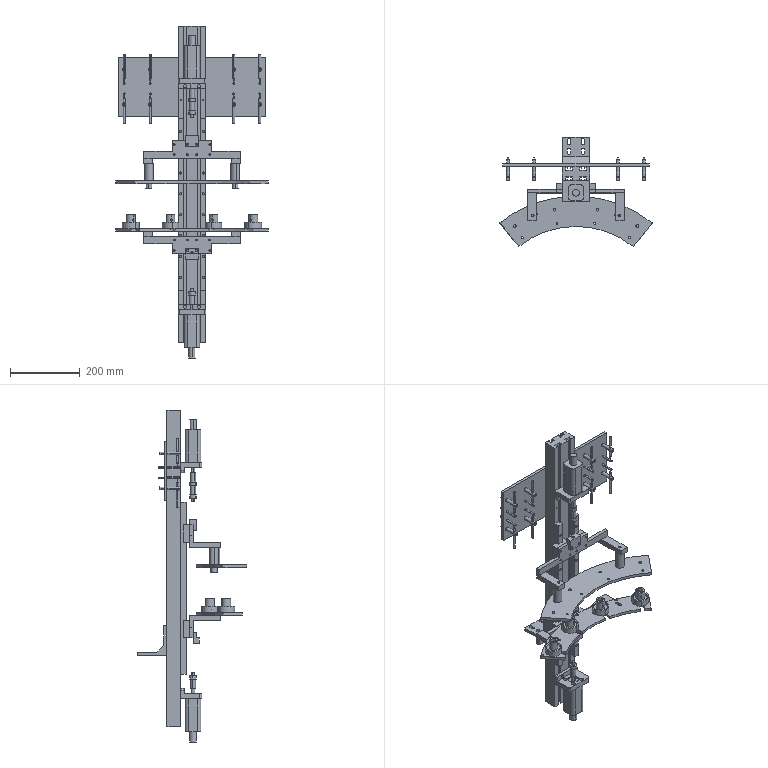Part | 54 solids | 1135 faces | box 437.882 x 314.149 x 954 mm | volume 4931479 mm3 | cylinder 648 | plane 369 | cone 118 | commonest cylinder face diameters 5 x96 3.3 x56 7 x42 5.5 x40 9 x40 6 x38